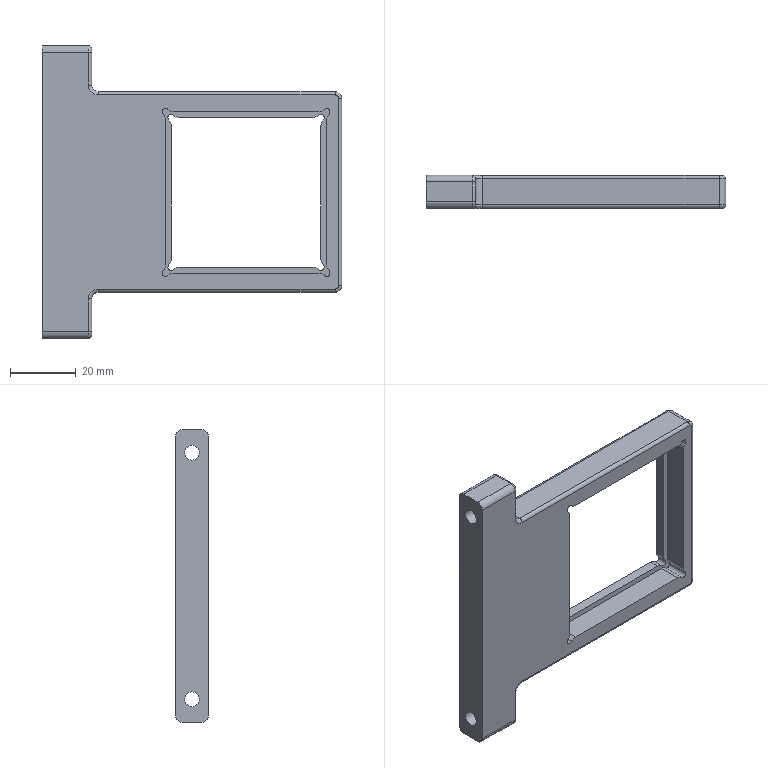NC program | NX | posted by the shop | part box 91 x 10 x 89 mm
Lines 1 to 38 of 16928:
%
O0001
(Machine time: 16.96 MIN)
(===Total Tool:8===)
(T1=D80R0.8 face mill D=80.  R=0.8  D-  H01 Z=0.    )
(T9=D10     D=10.  R=0.   D-  H09 Z=-10.2 )
(T4=D4      D=4.   R=0.   D-  H04 Z=-10.  )
(T11=D4-J   D=4.   R=0.   D-  H11 Z=-10.  )
(T19=D4R0.5 D=4.   R=0.5  D-  H19 Z=-2.5  )
(T2=D6 chamfer mill   D=6.   R=0.   D-  H02 Z=-1.5  )
(T17=D2-J   D=2.   R=0.   D-  H17 Z=-10.  )
(T10=D10-J  D=10.  R=0.   D10 H10 Z=-10.1 )
G80 G90 G17 G49 G40
G91 G28 Z0
M01
N1 T01 M06
(D80R0.8 face mill  D=80. R=0.8 H=01 ce=0.00 di=0.00)
G00 G90 G54 X90.5 Y-42.25 M03 S4000
G43 H01 Z20.
M08
Z2.
G01 Z0.0 F1000.
X85.5
X-85.5
Y0.0
X85.5
Y42.25
X-85.5
X-90.5
Z2.
G00 Z20.
G91 G28 Z0.0
M05
M09
G91 G28 Z0.0
M01